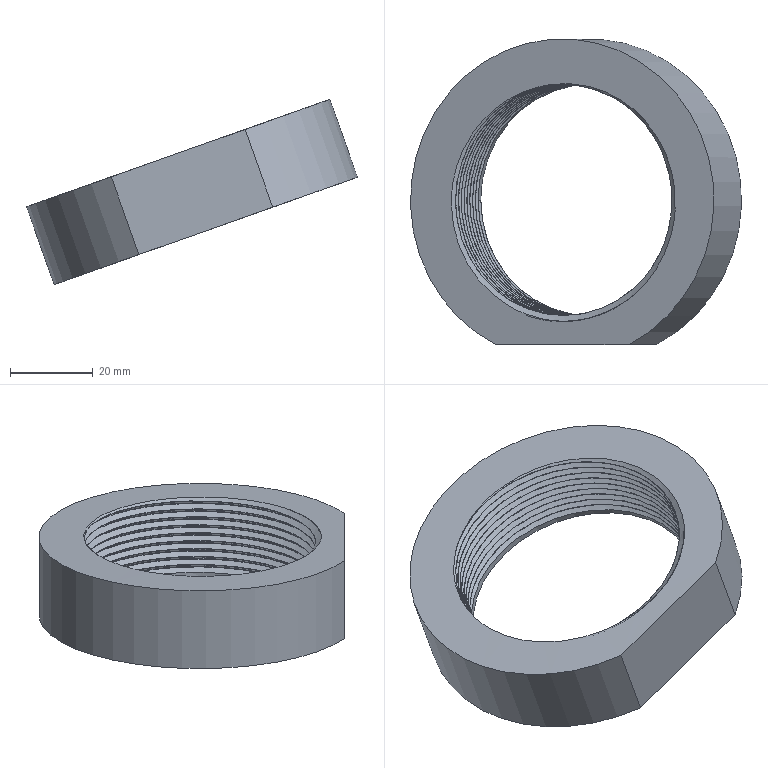Part | STEP file | SCREW-BUSH1_id522_x_t | 1 solid | 15 faces | box 80.202 x 74 x 44.89 mm | volume 42151 mm3 | spline 9 | plane 4 | cylinder 2 | commonest cylinder face diameters 56 x1 78 x1